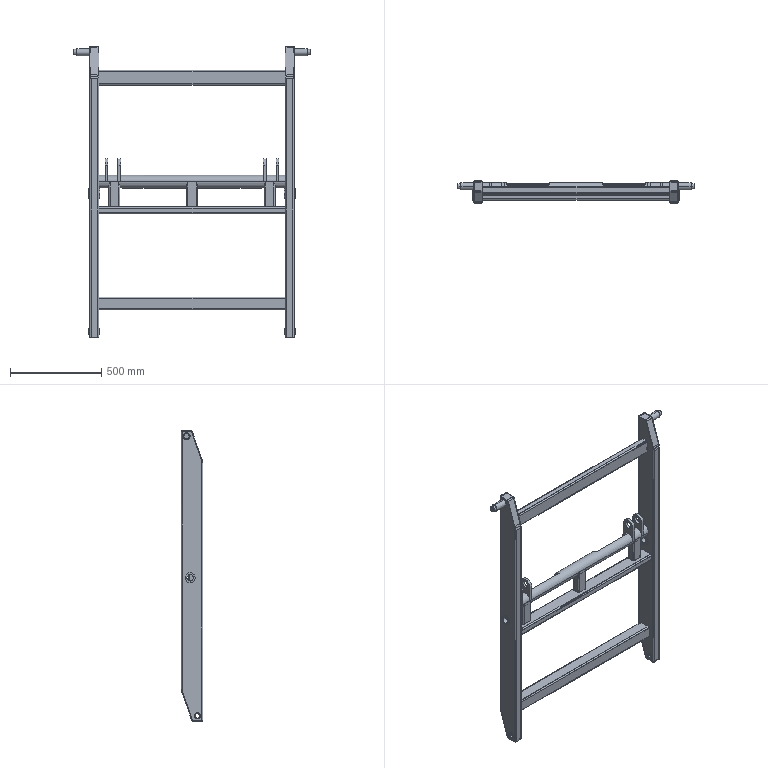Part | STEP file | BT2022003-01-05 Scissor beam A_Default<Machined> | 23 solids | 344 faces | box 1300 x 120 x 1590 mm | volume 10641393 mm3 | plane 171 | cylinder 165 | cone 8 | commonest cylinder face diameters 8 x48 16 x32 71 x13 20 x12 34 x12 55 x12